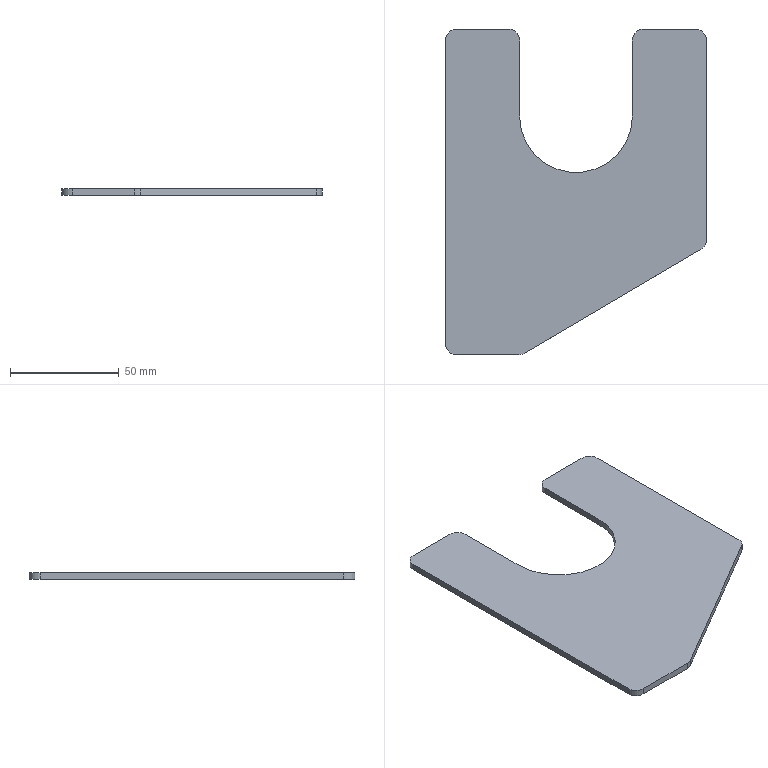Part | SolidWorks | features Extrusion 1 | 1 solid | 18 faces | box 120 x 150 x 3 mm | volume 38115 mm3 | plane 10 | cylinder 8 | commonest cylinder face diameters 10 x7 52 x1
STEP:
#1=CARTESIAN_POINT('',(86.,-40.,0.));
#2=VERTEX_POINT('',#1);
#3=CARTESIAN_POINT('',(34.,-40.,0.));
#4=VERTEX_POINT('',#3);
#5=CARTESIAN_POINT('',(60.,-40.,0.));
#6=DIRECTION('',(0.,0.,-1.));
#7=DIRECTION('',(1.,0.,0.));
#8=AXIS2_PLACEMENT_3D('',#5,#6,#7);
#9=CIRCLE('',#8,26.);
#10=EDGE_CURVE('',#2,#4,#9,.T.);
#11=ORIENTED_EDGE('',*,*,#10,.T.);
#12=CARTESIAN_POINT('',(34.,-40.,3.));
#13=VERTEX_POINT('',#12);
#14=CARTESIAN_POINT('',(34.,-40.,3.));
#15=DIRECTION('',(0.,0.,-1.));
#16=VECTOR('',#15,1000.);
#17=LINE('',#14,#16);
#18=EDGE_CURVE('',#13,#4,#17,.T.);
#19=ORIENTED_EDGE('',*,*,#18,.F.);
#20=CARTESIAN_POINT('',(86.,-40.,3.));
#21=VERTEX_POINT('',#20);
#22=CARTESIAN_POINT('',(60.,-40.,3.));
#23=DIRECTION('',(0.,0.,-1.));
#24=DIRECTION('',(1.,0.,0.));
#25=AXIS2_PLACEMENT_3D('',#22,#23,#24);
#26=CIRCLE('',#25,26.);
#27=EDGE_CURVE('',#21,#13,#26,.T.);
#28=ORIENTED_EDGE('',*,*,#27,.F.);
#29=CARTESIAN_POINT('',(86.,-40.,3.));
#30=DIRECTION('',(0.,0.,-1.));
#31=VECTOR('',#30,1000.);
#32=LINE('',#29,#31);
#33=EDGE_CURVE('',#21,#2,#32,.T.);
#34=ORIENTED_EDGE('',*,*,#33,.T.);
#35=EDGE_LOOP('',(#11,#19,#28,#34));
#36=FACE_OUTER_BOUND('',#35,.T.);
#37=CARTESIAN_POINT('',(60.,-40.,3.));
#38=DIRECTION('',(0.,0.,-1.));
#39=DIRECTION('',(-1.,0.,0.));
#40=AXIS2_PLACEMENT_3D('',#37,#38,#39);
#41=CYLINDRICAL_SURFACE('',#40,26.);
#42=ADVANCED_FACE('',(#36),#41,.F.);
#43=CARTESIAN_POINT('',(34.,-5.,0.));
#44=VERTEX_POINT('',#43);
#45=CARTESIAN_POINT('',(34.,-5.,0.));
#46=DIRECTION('',(0.,1.,0.));
#47=VECTOR('',#46,1000.);
#48=LINE('',#45,#47);
#49=EDGE_CURVE('',#4,#44,#48,.T.);
#50=ORIENTED_EDGE('',*,*,#49,.T.);
#51=CARTESIAN_POINT('',(34.,-5.,3.));
#52=VERTEX_POINT('',#51);
#53=CARTESIAN_POINT('',(34.,-5.,3.));
#54=DIRECTION('',(0.,0.,-1.));
#55=VECTOR('',#54,1000.);
#56=LINE('',#53,#55);
#57=EDGE_CURVE('',#52,#44,#56,.T.);
#58=ORIENTED_EDGE('',*,*,#57,.F.);
#59=CARTESIAN_POINT('',(34.,-5.,3.));
#60=DIRECTION('',(0.,1.,0.));
#61=VECTOR('',#60,1000.);
#62=LINE('',#59,#61);
#63=EDGE_CURVE('',#13,#52,#62,.T.);
#64=ORIENTED_EDGE('',*,*,#63,.F.);
#65=ORIENTED_EDGE('',*,*,#18,.T.);
#66=EDGE_LOOP('',(#50,#58,#64,#65));
#67=FACE_OUTER_BOUND('',#66,.T.);
#68=CARTESIAN_POINT('',(34.,-5.,3.));
#69=DIRECTION('',(-1.,0.,0.));
#70=DIRECTION('',(0.,-1.,0.));
#71=AXIS2_PLACEMENT_3D('',#68,#69,#70);
#72=PLANE('',#71);
#73=ADVANCED_FACE('',(#67),#72,.F.);
#74=CARTESIAN_POINT('',(29.,0.,0.));
#75=VERTEX_POINT('',#74);
#76=CARTESIAN_POINT('',(29.,-5.,0.));
#77=DIRECTION('',(0.,0.,1.));
#78=DIRECTION('',(1.,0.,0.));
#79=AXIS2_PLACEMENT_3D('',#76,#77,#78);
#80=CIRCLE('',#79,5.);
#81=EDGE_CURVE('',#44,#75,#80,.T.);
#82=ORIENTED_EDGE('',*,*,#81,.T.);
#83=CARTESIAN_POINT('',(29.,0.,3.));
#84=VERTEX_POINT('',#83);
#85=CARTESIAN_POINT('',(29.,0.,3.));
#86=DIRECTION('',(0.,0.,-1.));
#87=VECTOR('',#86,1000.);
#88=LINE('',#85,#87);
#89=EDGE_CURVE('',#84,#75,#88,.T.);
#90=ORIENTED_EDGE('',*,*,#89,.F.);
#91=CARTESIAN_POINT('',(29.,-5.,3.));
#92=DIRECTION('',(0.,0.,1.));
#93=DIRECTION('',(1.,0.,0.));
#94=AXIS2_PLACEMENT_3D('',#91,#92,#93);
#95=CIRCLE('',#94,5.);
#96=EDGE_CURVE('',#52,#84,#95,.T.);
#97=ORIENTED_EDGE('',*,*,#96,.F.);
#98=ORIENTED_EDGE('',*,*,#57,.T.);
#99=EDGE_LOOP('',(#82,#90,#97,#98));
#100=FACE_OUTER_BOUND('',#99,.T.);
#101=CARTESIAN_POINT('',(29.,-5.,3.));
#102=DIRECTION('',(0.,0.,-1.));
#103=DIRECTION('',(-1.,0.,0.));
#104=AXIS2_PLACEMENT_3D('',#101,#102,#103);
#105=CYLINDRICAL_SURFACE('',#104,5.);
#106=ADVANCED_FACE('',(#100),#105,.T.);
#107=CARTESIAN_POINT('',(5.,0.,0.));
#108=VERTEX_POINT('',#107);
#109=CARTESIAN_POINT('',(5.,0.,0.));
#110=DIRECTION('',(-1.,0.,0.));
#111=VECTOR('',#110,1000.);
#112=LINE('',#109,#111);
#113=EDGE_CURVE('',#75,#108,#112,.T.);
#114=ORIENTED_EDGE('',*,*,#113,.T.);
#115=CARTESIAN_POINT('',(5.,0.,3.));
#116=VERTEX_POINT('',#115);
#117=CARTESIAN_POINT('',(5.,0.,3.));
#118=DIRECTION('',(0.,0.,-1.));
#119=VECTOR('',#118,1000.);
#120=LINE('',#117,#119);
#121=EDGE_CURVE('',#116,#108,#120,.T.);
#122=ORIENTED_EDGE('',*,*,#121,.F.);
#123=CARTESIAN_POINT('',(5.,0.,3.));
#124=DIRECTION('',(-1.,0.,0.));
#125=VECTOR('',#124,1000.);
#126=LINE('',#123,#125);
#127=EDGE_CURVE('',#84,#116,#126,.T.);
#128=ORIENTED_EDGE('',*,*,#127,.F.);
#129=ORIENTED_EDGE('',*,*,#89,.T.);
#130=EDGE_LOOP('',(#114,#122,#128,#129));
#131=FACE_OUTER_BOUND('',#130,.T.);
#132=CARTESIAN_POINT('',(5.,0.,3.));
#133=DIRECTION('',(0.,-1.,0.));
#134=DIRECTION('',(0.,0.,-1.));
#135=AXIS2_PLACEMENT_3D('',#132,#133,#134);
#136=PLANE('',#135);
#137=ADVANCED_FACE('',(#131),#136,.F.);
#138=CARTESIAN_POINT('',(0.,-5.,0.));
#139=VERTEX_POINT('',#138);
#140=CARTESIAN_POINT('',(5.,-5.,0.));
#141=DIRECTION('',(0.,0.,1.));
#142=DIRECTION('',(-1.,0.,0.));
#143=AXIS2_PLACEMENT_3D('',#140,#141,#142);
#144=CIRCLE('',#143,5.);
#145=EDGE_CURVE('',#108,#139,#144,.T.);
#146=ORIENTED_EDGE('',*,*,#145,.T.);
#147=CARTESIAN_POINT('',(0.,-5.,3.));
#148=VERTEX_POINT('',#147);
#149=CARTESIAN_POINT('',(0.,-5.,3.));
#150=DIRECTION('',(0.,0.,-1.));
#151=VECTOR('',#150,1000.);
#152=LINE('',#149,#151);
#153=EDGE_CURVE('',#148,#139,#152,.T.);
#154=ORIENTED_EDGE('',*,*,#153,.F.);
#155=CARTESIAN_POINT('',(5.,-5.,3.));
#156=DIRECTION('',(0.,0.,1.));
#157=DIRECTION('',(-1.,0.,0.));
#158=AXIS2_PLACEMENT_3D('',#155,#156,#157);
#159=CIRCLE('',#158,5.);
#160=EDGE_CURVE('',#116,#148,#159,.T.);
#161=ORIENTED_EDGE('',*,*,#160,.F.);
#162=ORIENTED_EDGE('',*,*,#121,.T.);
#163=EDGE_LOOP('',(#146,#154,#161,#162));
#164=FACE_OUTER_BOUND('',#163,.T.);
#165=CARTESIAN_POINT('',(5.,-5.,3.));
#166=DIRECTION('',(0.,0.,-1.));
#167=DIRECTION('',(-1.,0.,0.));
#168=AXIS2_PLACEMENT_3D('',#165,#166,#167);
#169=CYLINDRICAL_SURFACE('',#168,5.);
#170=ADVANCED_FACE('',(#164),#169,.T.);
#171=CARTESIAN_POINT('',(0.,-145.,0.));
#172=VERTEX_POINT('',#171);
#173=CARTESIAN_POINT('',(0.,-5.,0.));
#174=DIRECTION('',(0.,-1.,0.));
#175=VECTOR('',#174,1000.);
#176=LINE('',#173,#175);
#177=EDGE_CURVE('',#139,#172,#176,.T.);
#178=ORIENTED_EDGE('',*,*,#177,.T.);
#179=CARTESIAN_POINT('',(0.,-145.,3.));
#180=VERTEX_POINT('',#179);
#181=CARTESIAN_POINT('',(0.,-145.,3.));
#182=DIRECTION('',(0.,0.,-1.));
#183=VECTOR('',#182,1000.);
#184=LINE('',#181,#183);
#185=EDGE_CURVE('',#180,#172,#184,.T.);
#186=ORIENTED_EDGE('',*,*,#185,.F.);
#187=CARTESIAN_POINT('',(0.,-5.,3.));
#188=DIRECTION('',(0.,-1.,0.));
#189=VECTOR('',#188,1000.);
#190=LINE('',#187,#189);
#191=EDGE_CURVE('',#148,#180,#190,.T.);
#192=ORIENTED_EDGE('',*,*,#191,.F.);
#193=ORIENTED_EDGE('',*,*,#153,.T.);
#194=EDGE_LOOP('',(#178,#186,#192,#193));
#195=FACE_OUTER_BOUND('',#194,.T.);
#196=CARTESIAN_POINT('',(0.,-5.,3.));
#197=DIRECTION('',(1.,0.,0.));
#198=DIRECTION('',(0.,0.,-1.));
#199=AXIS2_PLACEMENT_3D('',#196,#197,#198);
#200=PLANE('',#199);
#201=ADVANCED_FACE('',(#195),#200,.F.);
#202=CARTESIAN_POINT('',(5.,-150.,0.));
#203=VERTEX_POINT('',#202);
#204=CARTESIAN_POINT('',(5.,-145.,0.));
#205=DIRECTION('',(0.,0.,1.));
#206=DIRECTION('',(-1.,0.,0.));
#207=AXIS2_PLACEMENT_3D('',#204,#205,#206);
#208=CIRCLE('',#207,5.);
#209=EDGE_CURVE('',#172,#203,#208,.T.);
#210=ORIENTED_EDGE('',*,*,#209,.T.);
#211=CARTESIAN_POINT('',(5.,-150.,3.));
#212=VERTEX_POINT('',#211);
#213=CARTESIAN_POINT('',(5.,-150.,3.));
#214=DIRECTION('',(0.,0.,-1.));
#215=VECTOR('',#214,1000.);
#216=LINE('',#213,#215);
#217=EDGE_CURVE('',#212,#203,#216,.T.);
#218=ORIENTED_EDGE('',*,*,#217,.F.);
#219=CARTESIAN_POINT('',(5.,-145.,3.));
#220=DIRECTION('',(0.,0.,1.));
#221=DIRECTION('',(-1.,0.,0.));
#222=AXIS2_PLACEMENT_3D('',#219,#220,#221);
#223=CIRCLE('',#222,5.);
#224=EDGE_CURVE('',#180,#212,#223,.T.);
#225=ORIENTED_EDGE('',*,*,#224,.F.);
#226=ORIENTED_EDGE('',*,*,#185,.T.);
#227=EDGE_LOOP('',(#210,#218,#225,#226));
#228=FACE_OUTER_BOUND('',#227,.T.);
#229=CARTESIAN_POINT('',(5.,-145.,3.));
#230=DIRECTION('',(0.,0.,-1.));
#231=DIRECTION('',(-1.,0.,0.));
#232=AXIS2_PLACEMENT_3D('',#229,#230,#231);
#233=CYLINDRICAL_SURFACE('',#232,5.);
#234=ADVANCED_FACE('',(#228),#233,.T.);
#235=CARTESIAN_POINT('',(33.638,-150.,0.));
#236=VERTEX_POINT('',#235);
#237=CARTESIAN_POINT('',(5.,-150.,0.));
#238=DIRECTION('',(1.,0.,0.));
#239=VECTOR('',#238,1000.);
#240=LINE('',#237,#239);
#241=EDGE_CURVE('',#203,#236,#240,.T.);
#242=ORIENTED_EDGE('',*,*,#241,.T.);
#243=CARTESIAN_POINT('',(33.638,-150.,3.));
#244=VERTEX_POINT('',#243);
#245=CARTESIAN_POINT('',(33.638,-150.,3.));
#246=DIRECTION('',(0.,0.,-1.));
#247=VECTOR('',#246,1000.);
#248=LINE('',#245,#247);
#249=EDGE_CURVE('',#244,#236,#248,.T.);
#250=ORIENTED_EDGE('',*,*,#249,.F.);
#251=CARTESIAN_POINT('',(5.,-150.,3.));
#252=DIRECTION('',(1.,0.,0.));
#253=VECTOR('',#252,1000.);
#254=LINE('',#251,#253);
#255=EDGE_CURVE('',#212,#244,#254,.T.);
#256=ORIENTED_EDGE('',*,*,#255,.F.);
#257=ORIENTED_EDGE('',*,*,#217,.T.);
#258=EDGE_LOOP('',(#242,#250,#256,#257));
#259=FACE_OUTER_BOUND('',#258,.T.);
#260=CARTESIAN_POINT('',(5.,-150.,3.));
#261=DIRECTION('',(0.,1.,0.));
#262=DIRECTION('',(0.,0.,1.));
#263=AXIS2_PLACEMENT_3D('',#260,#261,#262);
#264=PLANE('',#263);
#265=ADVANCED_FACE('',(#259),#264,.F.);
#266=CARTESIAN_POINT('',(36.174,-149.31,0.));
#267=VERTEX_POINT('',#266);
#268=CARTESIAN_POINT('',(33.638,-145.,0.));
#269=DIRECTION('',(0.,0.,1.));
#270=DIRECTION('',(-1.,0.,0.));
#271=AXIS2_PLACEMENT_3D('',#268,#269,#270);
#272=CIRCLE('',#271,5.);
#273=EDGE_CURVE('',#236,#267,#272,.T.);
#274=ORIENTED_EDGE('',*,*,#273,.T.);
#275=CARTESIAN_POINT('',(36.174,-149.31,3.));
#276=VERTEX_POINT('',#275);
#277=CARTESIAN_POINT('',(36.174,-149.31,3.));
#278=DIRECTION('',(0.,0.,-1.));
#279=VECTOR('',#278,1000.);
#280=LINE('',#277,#279);
#281=EDGE_CURVE('',#276,#267,#280,.T.);
#282=ORIENTED_EDGE('',*,*,#281,.F.);
#283=CARTESIAN_POINT('',(33.638,-145.,3.));
#284=DIRECTION('',(0.,0.,1.));
#285=DIRECTION('',(-1.,0.,0.));
#286=AXIS2_PLACEMENT_3D('',#283,#284,#285);
#287=CIRCLE('',#286,5.);
#288=EDGE_CURVE('',#244,#276,#287,.T.);
#289=ORIENTED_EDGE('',*,*,#288,.F.);
#290=ORIENTED_EDGE('',*,*,#249,.T.);
#291=EDGE_LOOP('',(#274,#282,#289,#290));
#292=FACE_OUTER_BOUND('',#291,.T.);
#293=CARTESIAN_POINT('',(33.638,-145.,3.));
#294=DIRECTION('',(0.,0.,-1.));
#295=DIRECTION('',(-1.,0.,0.));
#296=AXIS2_PLACEMENT_3D('',#293,#294,#295);
#297=CYLINDRICAL_SURFACE('',#296,5.);
#298=ADVANCED_FACE('',(#292),#297,.T.);
#299=CARTESIAN_POINT('',(117.535,-101.45,0.));
#300=VERTEX_POINT('',#299);
#301=CARTESIAN_POINT('',(36.174,-149.31,0.));
#302=DIRECTION('',(0.8619,0.507,0.));
#303=VECTOR('',#302,1000.);
#304=LINE('',#301,#303);
#305=EDGE_CURVE('',#267,#300,#304,.T.);
#306=ORIENTED_EDGE('',*,*,#305,.T.);
#307=CARTESIAN_POINT('',(117.535,-101.45,3.));
#308=VERTEX_POINT('',#307);
#309=CARTESIAN_POINT('',(117.535,-101.45,3.));
#310=DIRECTION('',(0.,0.,-1.));
#311=VECTOR('',#310,1000.);
#312=LINE('',#309,#311);
#313=EDGE_CURVE('',#308,#300,#312,.T.);
#314=ORIENTED_EDGE('',*,*,#313,.F.);
#315=CARTESIAN_POINT('',(36.174,-149.31,3.));
#316=DIRECTION('',(0.8619,0.507,0.));
#317=VECTOR('',#316,1000.);
#318=LINE('',#315,#317);
#319=EDGE_CURVE('',#276,#308,#318,.T.);
#320=ORIENTED_EDGE('',*,*,#319,.F.);
#321=ORIENTED_EDGE('',*,*,#281,.T.);
#322=EDGE_LOOP('',(#306,#314,#320,#321));
#323=FACE_OUTER_BOUND('',#322,.T.);
#324=CARTESIAN_POINT('',(36.174,-149.31,3.));
#325=DIRECTION('',(-0.507,0.8619,0.));
#326=DIRECTION('',(-0.8619,-0.507,0.));
#327=AXIS2_PLACEMENT_3D('',#324,#325,#326);
#328=PLANE('',#327);
#329=ADVANCED_FACE('',(#323),#328,.F.);
#330=CARTESIAN_POINT('',(120.,-97.14,0.));
#331=VERTEX_POINT('',#330);
#332=CARTESIAN_POINT('',(115.,-97.14,0.));
#333=DIRECTION('',(0.,0.,1.));
#334=DIRECTION('',(-1.,0.,0.));
#335=AXIS2_PLACEMENT_3D('',#332,#333,#334);
#336=CIRCLE('',#335,5.);
#337=EDGE_CURVE('',#300,#331,#336,.T.);
#338=ORIENTED_EDGE('',*,*,#337,.T.);
#339=CARTESIAN_POINT('',(120.,-97.14,3.));
#340=VERTEX_POINT('',#339);
#341=CARTESIAN_POINT('',(120.,-97.14,3.));
#342=DIRECTION('',(0.,0.,-1.));
#343=VECTOR('',#342,1000.);
#344=LINE('',#341,#343);
#345=EDGE_CURVE('',#340,#331,#344,.T.);
#346=ORIENTED_EDGE('',*,*,#345,.F.);
#347=CARTESIAN_POINT('',(115.,-97.14,3.));
#348=DIRECTION('',(0.,0.,1.));
#349=DIRECTION('',(-1.,0.,0.));
#350=AXIS2_PLACEMENT_3D('',#347,#348,#349);
#351=CIRCLE('',#350,5.);
#352=EDGE_CURVE('',#308,#340,#351,.T.);
#353=ORIENTED_EDGE('',*,*,#352,.F.);
#354=ORIENTED_EDGE('',*,*,#313,.T.);
#355=EDGE_LOOP('',(#338,#346,#353,#354));
#356=FACE_OUTER_BOUND('',#355,.T.);
#357=CARTESIAN_POINT('',(115.,-97.14,3.));
#358=DIRECTION('',(0.,0.,-1.));
#359=DIRECTION('',(-1.,0.,0.));
#360=AXIS2_PLACEMENT_3D('',#357,#358,#359);
#361=CYLINDRICAL_SURFACE('',#360,5.);
#362=ADVANCED_FACE('',(#356),#361,.T.);
#363=CARTESIAN_POINT('',(120.,-5.,0.));
#364=VERTEX_POINT('',#363);
#365=CARTESIAN_POINT('',(120.,-97.14,0.));
#366=DIRECTION('',(0.,1.,0.));
#367=VECTOR('',#366,1000.);
#368=LINE('',#365,#367);
#369=EDGE_CURVE('',#331,#364,#368,.T.);
#370=ORIENTED_EDGE('',*,*,#369,.T.);
#371=CARTESIAN_POINT('',(120.,-5.,3.));
#372=VERTEX_POINT('',#371);
#373=CARTESIAN_POINT('',(120.,-5.,3.));
#374=DIRECTION('',(0.,0.,-1.));
#375=VECTOR('',#374,1000.);
#376=LINE('',#373,#375);
#377=EDGE_CURVE('',#372,#364,#376,.T.);
#378=ORIENTED_EDGE('',*,*,#377,.F.);
#379=CARTESIAN_POINT('',(120.,-97.14,3.));
#380=DIRECTION('',(0.,1.,0.));
#381=VECTOR('',#380,1000.);
#382=LINE('',#379,#381);
#383=EDGE_CURVE('',#340,#372,#382,.T.);
#384=ORIENTED_EDGE('',*,*,#383,.F.);
#385=ORIENTED_EDGE('',*,*,#345,.T.);
#386=EDGE_LOOP('',(#370,#378,#384,#385));
#387=FACE_OUTER_BOUND('',#386,.T.);
#388=CARTESIAN_POINT('',(120.,-97.14,3.));
#389=DIRECTION('',(-1.,0.,0.));
#390=DIRECTION('',(0.,-1.,0.));
#391=AXIS2_PLACEMENT_3D('',#388,#389,#390);
#392=PLANE('',#391);
#393=ADVANCED_FACE('',(#387),#392,.F.);
#394=CARTESIAN_POINT('',(115.,0.,0.));
#395=VERTEX_POINT('',#394);
#396=CARTESIAN_POINT('',(115.,-5.,0.));
#397=DIRECTION('',(0.,0.,1.));
#398=DIRECTION('',(-1.,0.,0.));
#399=AXIS2_PLACEMENT_3D('',#396,#397,#398);
#400=CIRCLE('',#399,5.);
#401=EDGE_CURVE('',#364,#395,#400,.T.);
#402=ORIENTED_EDGE('',*,*,#401,.T.);
#403=CARTESIAN_POINT('',(115.,0.,3.));
#404=VERTEX_POINT('',#403);
#405=CARTESIAN_POINT('',(115.,0.,3.));
#406=DIRECTION('',(0.,0.,-1.));
#407=VECTOR('',#406,1000.);
#408=LINE('',#405,#407);
#409=EDGE_CURVE('',#404,#395,#408,.T.);
#410=ORIENTED_EDGE('',*,*,#409,.F.);
#411=CARTESIAN_POINT('',(115.,-5.,3.));
#412=DIRECTION('',(0.,0.,1.));
#413=DIRECTION('',(-1.,0.,0.));
#414=AXIS2_PLACEMENT_3D('',#411,#412,#413);
#415=CIRCLE('',#414,5.);
#416=EDGE_CURVE('',#372,#404,#415,.T.);
#417=ORIENTED_EDGE('',*,*,#416,.F.);
#418=ORIENTED_EDGE('',*,*,#377,.T.);
#419=EDGE_LOOP('',(#402,#410,#417,#418));
#420=FACE_OUTER_BOUND('',#419,.T.);
#421=CARTESIAN_POINT('',(115.,-5.,3.));
#422=DIRECTION('',(0.,0.,-1.));
#423=DIRECTION('',(-1.,0.,0.));
#424=AXIS2_PLACEMENT_3D('',#421,#422,#423);
#425=CYLINDRICAL_SURFACE('',#424,5.);
#426=ADVANCED_FACE('',(#420),#425,.T.);
#427=CARTESIAN_POINT('',(91.,0.,0.));
#428=VERTEX_POINT('',#427);
#429=CARTESIAN_POINT('',(115.,0.,0.));
#430=DIRECTION('',(-1.,0.,0.));
#431=VECTOR('',#430,1000.);
#432=LINE('',#429,#431);
#433=EDGE_CURVE('',#395,#428,#432,.T.);
#434=ORIENTED_EDGE('',*,*,#433,.T.);
#435=CARTESIAN_POINT('',(91.,0.,3.));
#436=VERTEX_POINT('',#435);
#437=CARTESIAN_POINT('',(91.,0.,3.));
#438=DIRECTION('',(0.,0.,-1.));
#439=VECTOR('',#438,1000.);
#440=LINE('',#437,#439);
#441=EDGE_CURVE('',#436,#428,#440,.T.);
#442=ORIENTED_EDGE('',*,*,#441,.F.);
#443=CARTESIAN_POINT('',(115.,0.,3.));
#444=DIRECTION('',(-1.,0.,0.));
#445=VECTOR('',#444,1000.);
#446=LINE('',#443,#445);
#447=EDGE_CURVE('',#404,#436,#446,.T.);
#448=ORIENTED_EDGE('',*,*,#447,.F.);
#449=ORIENTED_EDGE('',*,*,#409,.T.);
#450=EDGE_LOOP('',(#434,#442,#448,#449));
#451=FACE_OUTER_BOUND('',#450,.T.);
#452=CARTESIAN_POINT('',(115.,0.,3.));
#453=DIRECTION('',(0.,-1.,0.));
#454=DIRECTION('',(1.,0.,0.));
#455=AXIS2_PLACEMENT_3D('',#452,#453,#454);
#456=PLANE('',#455);
#457=ADVANCED_FACE('',(#451),#456,.F.);
#458=CARTESIAN_POINT('',(86.,-5.,0.));
#459=VERTEX_POINT('',#458);
#460=CARTESIAN_POINT('',(91.,-5.,0.));
#461=DIRECTION('',(0.,0.,1.));
#462=DIRECTION('',(1.,0.,0.));
#463=AXIS2_PLACEMENT_3D('',#460,#461,#462);
#464=CIRCLE('',#463,5.);
#465=EDGE_CURVE('',#428,#459,#464,.T.);
#466=ORIENTED_EDGE('',*,*,#465,.T.);
#467=CARTESIAN_POINT('',(86.,-5.,3.));
#468=VERTEX_POINT('',#467);
#469=CARTESIAN_POINT('',(86.,-5.,3.));
#470=DIRECTION('',(0.,0.,-1.));
#471=VECTOR('',#470,1000.);
#472=LINE('',#469,#471);
#473=EDGE_CURVE('',#468,#459,#472,.T.);
#474=ORIENTED_EDGE('',*,*,#473,.F.);
#475=CARTESIAN_POINT('',(91.,-5.,3.));
#476=DIRECTION('',(0.,0.,1.));
#477=DIRECTION('',(1.,0.,0.));
#478=AXIS2_PLACEMENT_3D('',#475,#476,#477);
#479=CIRCLE('',#478,5.);
#480=EDGE_CURVE('',#436,#468,#479,.T.);
#481=ORIENTED_EDGE('',*,*,#480,.F.);
#482=ORIENTED_EDGE('',*,*,#441,.T.);
#483=EDGE_LOOP('',(#466,#474,#481,#482));
#484=FACE_OUTER_BOUND('',#483,.T.);
#485=CARTESIAN_POINT('',(91.,-5.,3.));
#486=DIRECTION('',(0.,0.,-1.));
#487=DIRECTION('',(-1.,0.,0.));
#488=AXIS2_PLACEMENT_3D('',#485,#486,#487);
#489=CYLINDRICAL_SURFACE('',#488,5.);
#490=ADVANCED_FACE('',(#484),#489,.T.);
#491=CARTESIAN_POINT('',(86.,-5.,0.));
#492=DIRECTION('',(0.,-1.,0.));
#493=VECTOR('',#492,1000.);
#494=LINE('',#491,#493);
#495=EDGE_CURVE('',#459,#2,#494,.T.);
#496=ORIENTED_EDGE('',*,*,#495,.T.);
#497=ORIENTED_EDGE('',*,*,#33,.F.);
#498=CARTESIAN_POINT('',(86.,-5.,3.));
#499=DIRECTION('',(0.,-1.,0.));
#500=VECTOR('',#499,1000.);
#501=LINE('',#498,#500);
#502=EDGE_CURVE('',#468,#21,#501,.T.);
#503=ORIENTED_EDGE('',*,*,#502,.F.);
#504=ORIENTED_EDGE('',*,*,#473,.T.);
#505=EDGE_LOOP('',(#496,#497,#503,#504));
#506=FACE_OUTER_BOUND('',#505,.T.);
#507=CARTESIAN_POINT('',(86.,-5.,3.));
#508=DIRECTION('',(1.,0.,0.));
#509=DIRECTION('',(0.,0.,-1.));
#510=AXIS2_PLACEMENT_3D('',#507,#508,#509);
#511=PLANE('',#510);
#512=ADVANCED_FACE('',(#506),#511,.F.);
#513=ORIENTED_EDGE('',*,*,#27,.T.);
#514=ORIENTED_EDGE('',*,*,#63,.T.);
#515=ORIENTED_EDGE('',*,*,#96,.T.);
#516=ORIENTED_EDGE('',*,*,#127,.T.);
#517=ORIENTED_EDGE('',*,*,#160,.T.);
#518=ORIENTED_EDGE('',*,*,#191,.T.);
#519=ORIENTED_EDGE('',*,*,#224,.T.);
#520=ORIENTED_EDGE('',*,*,#255,.T.);
#521=ORIENTED_EDGE('',*,*,#288,.T.);
#522=ORIENTED_EDGE('',*,*,#319,.T.);
#523=ORIENTED_EDGE('',*,*,#352,.T.);
#524=ORIENTED_EDGE('',*,*,#383,.T.);
#525=ORIENTED_EDGE('',*,*,#416,.T.);
#526=ORIENTED_EDGE('',*,*,#447,.T.);
#527=ORIENTED_EDGE('',*,*,#480,.T.);
#528=ORIENTED_EDGE('',*,*,#502,.T.);
#529=EDGE_LOOP('',(#513,#514,#515,#516,#517,#518,#519,#520,#521,#522,#523,#524,#525,#526,#527,#528));
#530=FACE_OUTER_BOUND('',#529,.T.);
#531=CARTESIAN_POINT('',(60.,-40.,3.));
#532=DIRECTION('',(0.,0.,1.));
#533=DIRECTION('',(1.,0.,0.));
#534=AXIS2_PLACEMENT_3D('',#531,#532,#533);
#535=PLANE('',#534);
#536=ADVANCED_FACE('',(#530),#535,.T.);
#537=ORIENTED_EDGE('',*,*,#10,.F.);
#538=ORIENTED_EDGE('',*,*,#495,.F.);
#539=ORIENTED_EDGE('',*,*,#465,.F.);
#540=ORIENTED_EDGE('',*,*,#433,.F.);
#541=ORIENTED_EDGE('',*,*,#401,.F.);
#542=ORIENTED_EDGE('',*,*,#369,.F.);
#543=ORIENTED_EDGE('',*,*,#337,.F.);
#544=ORIENTED_EDGE('',*,*,#305,.F.);
#545=ORIENTED_EDGE('',*,*,#273,.F.);
#546=ORIENTED_EDGE('',*,*,#241,.F.);
#547=ORIENTED_EDGE('',*,*,#209,.F.);
#548=ORIENTED_EDGE('',*,*,#177,.F.);
#549=ORIENTED_EDGE('',*,*,#145,.F.);
#550=ORIENTED_EDGE('',*,*,#113,.F.);
#551=ORIENTED_EDGE('',*,*,#81,.F.);
#552=ORIENTED_EDGE('',*,*,#49,.F.);
#553=EDGE_LOOP('',(#537,#538,#539,#540,#541,#542,#543,#544,#545,#546,#547,#548,#549,#550,#551,#552));
#554=FACE_OUTER_BOUND('',#553,.T.);
#555=CARTESIAN_POINT('',(60.,-40.,0.));
#556=DIRECTION('',(0.,0.,1.));
#557=DIRECTION('',(1.,0.,0.));
#558=AXIS2_PLACEMENT_3D('',#555,#556,#557);
#559=PLANE('',#558);
#560=ADVANCED_FACE('',(#554),#559,.F.);
#561=CLOSED_SHELL('',(#42,#73,#106,#137,#170,#201,#234,#265,#298,#329,#362,#393,#426,#457,#490,#512,#536,#560));
#562=MANIFOLD_SOLID_BREP('',#561);
#563=CARTESIAN_POINT('',(0.,0.,0.));
#564=DIRECTION('',(0.,0.,1.));
#565=DIRECTION('',(1.,0.,0.));
#566=AXIS2_PLACEMENT_3D('',#563,#564,#565);
#567=(LENGTH_UNIT()NAMED_UNIT(*)SI_UNIT(.MILLI.,.METRE.));
#568=UNCERTAINTY_MEASURE_WITH_UNIT(LENGTH_MEASURE(0.00001),#567,'','');
#569=(NAMED_UNIT(*)PLANE_ANGLE_UNIT()SI_UNIT($,.RADIAN.));
#570=(NAMED_UNIT(*)SI_UNIT($,.STERADIAN.)SOLID_ANGLE_UNIT());
#571=(GEOMETRIC_REPRESENTATION_CONTEXT(3)GLOBAL_UNCERTAINTY_ASSIGNED_CONTEXT((#568))GLOBAL_UNIT_ASSIGNED_CONTEXT((#567,#569,#570))REPRESENTATION_CONTEXT('',''));
#572=ADVANCED_BREP_SHAPE_REPRESENTATION('',(#562,#566),#571);